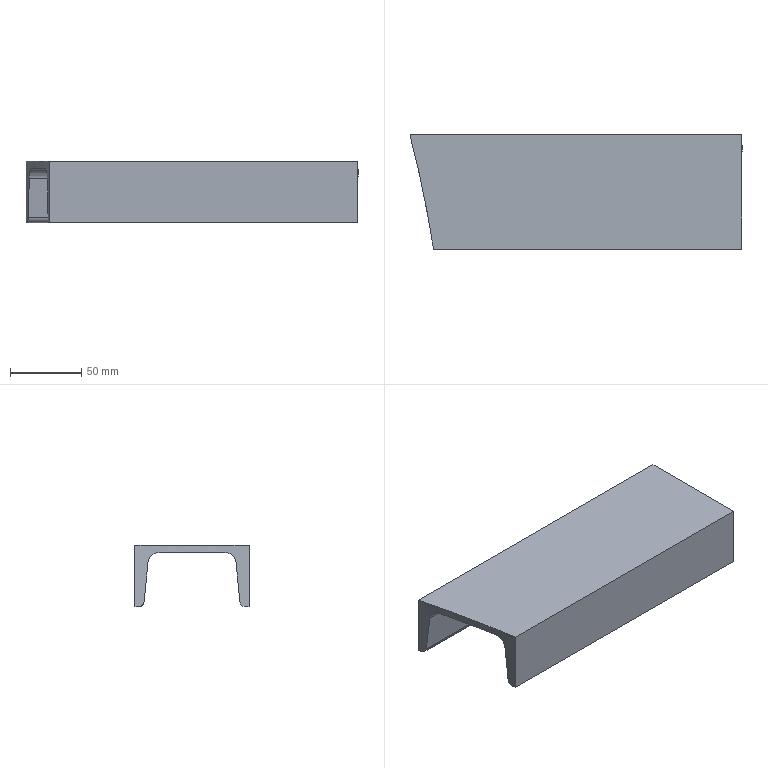Part | SolidWorks | features ICE 2, WeldMemberFeat 1, WeldmentFeature 1 | 1 solid | 14 faces | box 232.5 x 80 x 43 mm | volume 229319 mm3 | plane 9 | cylinder 5 | commonest cylinder face diameters 8 x2 16 x2 1790 x1
STEP:
#1=CARTESIAN_POINT('',(83.602,-77.52,-43.));
#2=VERTEX_POINT('',#1);
#3=CARTESIAN_POINT('',(82.948,-73.54,-39.398));
#4=VERTEX_POINT('',#3);
#5=CARTESIAN_POINT('',(83.602,-77.52,-43.));
#6=CARTESIAN_POINT('',(83.562,-77.274,-43.));
#7=CARTESIAN_POINT('',(83.523,-77.032,-42.978));
#8=CARTESIAN_POINT('',(83.445,-76.555,-42.889));
#9=CARTESIAN_POINT('',(83.407,-76.318,-42.823));
#10=CARTESIAN_POINT('',(83.332,-75.86,-42.648));
#11=CARTESIAN_POINT('',(83.296,-75.642,-42.54));
#12=CARTESIAN_POINT('',(83.227,-75.227,-42.286));
#13=CARTESIAN_POINT('',(83.195,-75.028,-42.138));
#14=CARTESIAN_POINT('',(83.134,-74.663,-41.81));
#15=CARTESIAN_POINT('',(83.107,-74.497,-41.631));
#16=CARTESIAN_POINT('',(83.058,-74.199,-41.242));
#17=CARTESIAN_POINT('',(83.036,-74.065,-41.031));
#18=CARTESIAN_POINT('',(82.998,-73.842,-40.592));
#19=CARTESIAN_POINT('',(82.983,-73.752,-40.365));
#20=CARTESIAN_POINT('',(82.96,-73.613,-39.892));
#21=CARTESIAN_POINT('',(82.952,-73.565,-39.646));
#22=CARTESIAN_POINT('',(82.948,-73.54,-39.398));
#23=B_SPLINE_CURVE_WITH_KNOTS('',3,(#5,#6,#7,#8,#9,#10,#11,#12,#13,#14,#15,#16,#17,#18,#19,#20,#21,#22),.UNSPECIFIED.,.F.,.F.,(4,2,2,2,2,2,2,2,4),(0.,0.0007369,0.001474,0.002211,0.002947,0.003684,0.004421,0.005158,0.005895),.UNSPECIFIED.);
#24=EDGE_CURVE('',#2,#4,#23,.T.);
#25=ORIENTED_EDGE('',*,*,#24,.T.);
#26=CARTESIAN_POINT('',(300.,-73.54,-39.398));
#27=VERTEX_POINT('',#26);
#28=CARTESIAN_POINT('',(300.,-73.54,-39.398));
#29=DIRECTION('',(-1.,0.,0.));
#30=VECTOR('',#29,1000.);
#31=LINE('',#28,#30);
#32=EDGE_CURVE('',#27,#4,#31,.T.);
#33=ORIENTED_EDGE('',*,*,#32,.F.);
#34=CARTESIAN_POINT('',(300.,-77.52,-43.));
#35=VERTEX_POINT('',#34);
#36=CARTESIAN_POINT('',(300.,-77.52,-39.));
#37=DIRECTION('',(-1.,0.,0.));
#38=DIRECTION('',(0.,1.,0.));
#39=AXIS2_PLACEMENT_3D('',#36,#37,#38);
#40=CIRCLE('',#39,4.);
#41=EDGE_CURVE('',#27,#35,#40,.T.);
#42=ORIENTED_EDGE('',*,*,#41,.T.);
#43=CARTESIAN_POINT('',(300.,-77.52,-43.));
#44=DIRECTION('',(-1.,0.,0.));
#45=VECTOR('',#44,1000.);
#46=LINE('',#43,#45);
#47=EDGE_CURVE('',#35,#2,#46,.T.);
#48=ORIENTED_EDGE('',*,*,#47,.T.);
#49=EDGE_LOOP('',(#25,#33,#42,#48));
#50=FACE_OUTER_BOUND('',#49,.T.);
#51=CARTESIAN_POINT('',(300.,-77.52,-39.));
#52=DIRECTION('',(-1.,0.,0.));
#53=DIRECTION('',(0.,0.,1.));
#54=AXIS2_PLACEMENT_3D('',#51,#52,#53);
#55=CYLINDRICAL_SURFACE('',#54,4.);
#56=ADVANCED_FACE('',(#50),#55,.T.);
#57=CARTESIAN_POINT('',(82.491,-70.82,-12.204));
#58=VERTEX_POINT('',#57);
#59=CARTESIAN_POINT('',(82.948,-73.54,-39.398));
#60=CARTESIAN_POINT('',(82.797,-72.633,-30.331));
#61=CARTESIAN_POINT('',(82.645,-71.727,-21.266));
#62=CARTESIAN_POINT('',(82.491,-70.82,-12.204));
#63=(BOUNDED_CURVE()B_SPLINE_CURVE(3,(#59,#60,#61,#62),.UNSPECIFIED.,.F.,.F.)B_SPLINE_CURVE_WITH_KNOTS((4,4),(4.877,4.881),.UNSPECIFIED.)CURVE()GEOMETRIC_REPRESENTATION_ITEM()RATIONAL_B_SPLINE_CURVE((1.,1.,1.,1.))REPRESENTATION_ITEM(''));
#64=EDGE_CURVE('',#4,#58,#63,.T.);
#65=ORIENTED_EDGE('',*,*,#64,.T.);
#66=CARTESIAN_POINT('',(300.,-70.82,-12.204));
#67=VERTEX_POINT('',#66);
#68=CARTESIAN_POINT('',(300.,-70.82,-12.204));
#69=DIRECTION('',(-1.,0.,0.));
#70=VECTOR('',#69,1000.);
#71=LINE('',#68,#70);
#72=EDGE_CURVE('',#67,#58,#71,.T.);
#73=ORIENTED_EDGE('',*,*,#72,.F.);
#74=CARTESIAN_POINT('',(300.,-70.82,-12.204));
#75=DIRECTION('',(0.,-0.0995,-0.995));
#76=VECTOR('',#75,1000.);
#77=LINE('',#74,#76);
#78=EDGE_CURVE('',#67,#27,#77,.T.);
#79=ORIENTED_EDGE('',*,*,#78,.T.);
#80=ORIENTED_EDGE('',*,*,#32,.T.);
#81=EDGE_LOOP('',(#65,#73,#79,#80));
#82=FACE_OUTER_BOUND('',#81,.T.);
#83=CARTESIAN_POINT('',(300.,-70.82,-12.204));
#84=DIRECTION('',(0.,0.995,-0.0995));
#85=DIRECTION('',(0.,0.0995,0.995));
#86=AXIS2_PLACEMENT_3D('',#83,#84,#85);
#87=PLANE('',#86);
#88=ADVANCED_FACE('',(#82),#87,.T.);
#89=CARTESIAN_POINT('',(81.103,-62.86,-5.));
#90=VERTEX_POINT('',#89);
#91=CARTESIAN_POINT('',(82.491,-70.82,-12.204));
#92=CARTESIAN_POINT('',(82.482,-70.771,-11.708));
#93=CARTESIAN_POINT('',(82.466,-70.676,-11.224));
#94=CARTESIAN_POINT('',(82.431,-70.469,-10.517));
#95=CARTESIAN_POINT('',(82.418,-70.389,-10.284));
#96=CARTESIAN_POINT('',(82.387,-70.207,-9.825));
#97=CARTESIAN_POINT('',(82.369,-70.105,-9.598));
#98=CARTESIAN_POINT('',(82.312,-69.769,-8.936));
#99=CARTESIAN_POINT('',(82.267,-69.507,-8.522));
#100=CARTESIAN_POINT('',(82.19,-69.061,-7.939));
#101=CARTESIAN_POINT('',(82.163,-68.902,-7.751));
#102=CARTESIAN_POINT('',(82.105,-68.567,-7.388));
#103=CARTESIAN_POINT('',(82.075,-68.391,-7.215));
#104=CARTESIAN_POINT('',(81.981,-67.844,-6.723));
#105=CARTESIAN_POINT('',(81.913,-67.454,-6.432));
#106=CARTESIAN_POINT('',(81.768,-66.621,-5.922));
#107=CARTESIAN_POINT('',(81.69,-66.176,-5.703));
#108=CARTESIAN_POINT('',(81.53,-65.268,-5.355));
#109=CARTESIAN_POINT('',(81.448,-64.801,-5.224));
#110=CARTESIAN_POINT('',(81.278,-63.842,-5.046));
#111=CARTESIAN_POINT('',(81.19,-63.351,-5.));
#112=CARTESIAN_POINT('',(81.103,-62.86,-5.));
#113=B_SPLINE_CURVE_WITH_KNOTS('',3,(#91,#92,#93,#94,#95,#96,#97,#98,#99,#100,#101,#102,#103,#104,#105,#106,#107,#108,#109,#110,#111,#112),.UNSPECIFIED.,.F.,.F.,(4,2,2,2,2,2,2,2,2,2,4),(0.,0.001475,0.002212,0.00295,0.004425,0.005162,0.0059,0.007375,0.00885,0.01032,0.0118),.UNSPECIFIED.);
#114=EDGE_CURVE('',#58,#90,#113,.T.);
#115=ORIENTED_EDGE('',*,*,#114,.T.);
#116=CARTESIAN_POINT('',(300.,-62.86,-5.));
#117=VERTEX_POINT('',#116);
#118=CARTESIAN_POINT('',(300.,-62.86,-5.));
#119=DIRECTION('',(-1.,0.,0.));
#120=VECTOR('',#119,1000.);
#121=LINE('',#118,#120);
#122=EDGE_CURVE('',#117,#90,#121,.T.);
#123=ORIENTED_EDGE('',*,*,#122,.F.);
#124=CARTESIAN_POINT('',(300.,-62.86,-13.));
#125=DIRECTION('',(1.,0.,0.));
#126=DIRECTION('',(0.,-1.,0.));
#127=AXIS2_PLACEMENT_3D('',#124,#125,#126);
#128=CIRCLE('',#127,8.);
#129=EDGE_CURVE('',#117,#67,#128,.T.);
#130=ORIENTED_EDGE('',*,*,#129,.T.);
#131=ORIENTED_EDGE('',*,*,#72,.T.);
#132=EDGE_LOOP('',(#115,#123,#130,#131));
#133=FACE_OUTER_BOUND('',#132,.T.);
#134=CARTESIAN_POINT('',(300.,-62.86,-13.));
#135=DIRECTION('',(-1.,0.,0.));
#136=DIRECTION('',(0.,0.,1.));
#137=AXIS2_PLACEMENT_3D('',#134,#135,#136);
#138=CYLINDRICAL_SURFACE('',#137,8.);
#139=ADVANCED_FACE('',(#133),#138,.F.);
#140=CARTESIAN_POINT('',(71.68,-17.14,-5.));
#141=VERTEX_POINT('',#140);
#142=CARTESIAN_POINT('',(-799.887,-220.6,-5.));
#143=DIRECTION('',(0.,0.,1.));
#144=DIRECTION('',(0.,1.,0.));
#145=AXIS2_PLACEMENT_3D('',#142,#143,#144);
#146=CIRCLE('',#145,895.);
#147=EDGE_CURVE('',#90,#141,#146,.T.);
#148=ORIENTED_EDGE('',*,*,#147,.T.);
#149=CARTESIAN_POINT('',(300.,-17.14,-5.));
#150=VERTEX_POINT('',#149);
#151=CARTESIAN_POINT('',(300.,-17.14,-5.));
#152=DIRECTION('',(-1.,0.,0.));
#153=VECTOR('',#152,1000.);
#154=LINE('',#151,#153);
#155=EDGE_CURVE('',#150,#141,#154,.T.);
#156=ORIENTED_EDGE('',*,*,#155,.F.);
#157=CARTESIAN_POINT('',(300.,-62.86,-5.));
#158=DIRECTION('',(0.,-1.,0.));
#159=VECTOR('',#158,1000.);
#160=LINE('',#157,#159);
#161=EDGE_CURVE('',#150,#117,#160,.T.);
#162=ORIENTED_EDGE('',*,*,#161,.T.);
#163=ORIENTED_EDGE('',*,*,#122,.T.);
#164=EDGE_LOOP('',(#148,#156,#162,#163));
#165=FACE_OUTER_BOUND('',#164,.T.);
#166=CARTESIAN_POINT('',(300.,-62.86,-5.));
#167=DIRECTION('',(0.,0.,-1.));
#168=DIRECTION('',(0.,1.,0.));
#169=AXIS2_PLACEMENT_3D('',#166,#167,#168);
#170=PLANE('',#169);
#171=ADVANCED_FACE('',(#165),#170,.T.);
#172=CARTESIAN_POINT('',(69.783,-9.18,-12.204));
#173=VERTEX_POINT('',#172);
#174=CARTESIAN_POINT('',(71.68,-17.14,-5.));
#175=CARTESIAN_POINT('',(71.566,-16.651,-5.));
#176=CARTESIAN_POINT('',(71.453,-16.169,-5.044));
#177=CARTESIAN_POINT('',(71.285,-15.458,-5.175));
#178=CARTESIAN_POINT('',(71.23,-15.222,-5.229));
#179=CARTESIAN_POINT('',(71.12,-14.755,-5.36));
#180=CARTESIAN_POINT('',(71.065,-14.522,-5.436));
#181=CARTESIAN_POINT('',(70.902,-13.837,-5.697));
#182=CARTESIAN_POINT('',(70.799,-13.401,-5.911));
#183=CARTESIAN_POINT('',(70.65,-12.78,-6.288));
#184=CARTESIAN_POINT('',(70.602,-12.577,-6.424));
#185=CARTESIAN_POINT('',(70.508,-12.184,-6.715));
#186=CARTESIAN_POINT('',(70.462,-11.992,-6.872));
#187=CARTESIAN_POINT('',(70.33,-11.442,-7.363));
#188=CARTESIAN_POINT('',(70.25,-11.109,-7.721));
#189=CARTESIAN_POINT('',(70.142,-10.66,-8.302));
#190=CARTESIAN_POINT('',(70.107,-10.518,-8.504));
#191=CARTESIAN_POINT('',(70.043,-10.253,-8.922));
#192=CARTESIAN_POINT('',(70.013,-10.129,-9.14));
#193=CARTESIAN_POINT('',(69.931,-9.791,-9.801));
#194=CARTESIAN_POINT('',(69.887,-9.608,-10.259));
#195=CARTESIAN_POINT('',(69.819,-9.327,-11.209));
#196=CARTESIAN_POINT('',(69.795,-9.23,-11.704));
#197=CARTESIAN_POINT('',(69.783,-9.18,-12.204));
#198=B_SPLINE_CURVE_WITH_KNOTS('',3,(#174,#175,#176,#177,#178,#179,#180,#181,#182,#183,#184,#185,#186,#187,#188,#189,#190,#191,#192,#193,#194,#195,#196,#197),.UNSPECIFIED.,.F.,.F.,(4,2,2,2,2,2,2,2,2,2,2,4),(0.,0.001485,0.002228,0.00297,0.004456,0.005198,0.005941,0.007426,0.008169,0.008911,0.0104,0.01188),.UNSPECIFIED.);
#199=EDGE_CURVE('',#141,#173,#198,.T.);
#200=ORIENTED_EDGE('',*,*,#199,.T.);
#201=CARTESIAN_POINT('',(300.,-9.18,-12.204));
#202=VERTEX_POINT('',#201);
#203=CARTESIAN_POINT('',(300.,-9.18,-12.204));
#204=DIRECTION('',(-1.,0.,0.));
#205=VECTOR('',#204,1000.);
#206=LINE('',#203,#205);
#207=EDGE_CURVE('',#202,#173,#206,.T.);
#208=ORIENTED_EDGE('',*,*,#207,.F.);
#209=CARTESIAN_POINT('',(300.,-17.14,-13.));
#210=DIRECTION('',(1.,0.,0.));
#211=DIRECTION('',(0.,1.,0.));
#212=AXIS2_PLACEMENT_3D('',#209,#210,#211);
#213=CIRCLE('',#212,8.);
#214=EDGE_CURVE('',#202,#150,#213,.T.);
#215=ORIENTED_EDGE('',*,*,#214,.T.);
#216=ORIENTED_EDGE('',*,*,#155,.T.);
#217=EDGE_LOOP('',(#200,#208,#215,#216));
#218=FACE_OUTER_BOUND('',#217,.T.);
#219=CARTESIAN_POINT('',(300.,-17.14,-13.));
#220=DIRECTION('',(-1.,0.,0.));
#221=DIRECTION('',(0.,0.,1.));
#222=AXIS2_PLACEMENT_3D('',#219,#220,#221);
#223=CYLINDRICAL_SURFACE('',#222,8.);
#224=ADVANCED_FACE('',(#218),#223,.F.);
#225=CARTESIAN_POINT('',(69.117,-6.46,-39.398));
#226=VERTEX_POINT('',#225);
#227=CARTESIAN_POINT('',(69.783,-9.18,-12.204));
#228=CARTESIAN_POINT('',(69.563,-8.273,-21.272));
#229=CARTESIAN_POINT('',(69.341,-7.366,-30.337));
#230=CARTESIAN_POINT('',(69.117,-6.46,-39.398));
#231=(BOUNDED_CURVE()B_SPLINE_CURVE(3,(#227,#228,#229,#230),.UNSPECIFIED.,.F.,.F.)B_SPLINE_CURVE_WITH_KNOTS((4,4),(1.809,1.812),.UNSPECIFIED.)CURVE()GEOMETRIC_REPRESENTATION_ITEM()RATIONAL_B_SPLINE_CURVE((1.,1.,1.,1.))REPRESENTATION_ITEM(''));
#232=EDGE_CURVE('',#173,#226,#231,.T.);
#233=ORIENTED_EDGE('',*,*,#232,.T.);
#234=CARTESIAN_POINT('',(300.,-6.46,-39.398));
#235=VERTEX_POINT('',#234);
#236=CARTESIAN_POINT('',(300.,-6.46,-39.398));
#237=DIRECTION('',(-1.,0.,0.));
#238=VECTOR('',#237,1000.);
#239=LINE('',#236,#238);
#240=EDGE_CURVE('',#235,#226,#239,.T.);
#241=ORIENTED_EDGE('',*,*,#240,.F.);
#242=CARTESIAN_POINT('',(300.,-9.18,-12.204));
#243=DIRECTION('',(0.,-0.0995,0.995));
#244=VECTOR('',#243,1000.);
#245=LINE('',#242,#244);
#246=EDGE_CURVE('',#235,#202,#245,.T.);
#247=ORIENTED_EDGE('',*,*,#246,.T.);
#248=ORIENTED_EDGE('',*,*,#207,.T.);
#249=EDGE_LOOP('',(#233,#241,#247,#248));
#250=FACE_OUTER_BOUND('',#249,.T.);
#251=CARTESIAN_POINT('',(300.,-9.18,-12.204));
#252=DIRECTION('',(0.,-0.995,-0.0995));
#253=DIRECTION('',(0.,0.0995,-0.995));
#254=AXIS2_PLACEMENT_3D('',#251,#252,#253);
#255=PLANE('',#254);
#256=ADVANCED_FACE('',(#250),#255,.T.);
#257=CARTESIAN_POINT('',(68.127,-2.48,-43.));
#258=VERTEX_POINT('',#257);
#259=CARTESIAN_POINT('',(69.117,-6.46,-39.398));
#260=CARTESIAN_POINT('',(69.111,-6.435,-39.648));
#261=CARTESIAN_POINT('',(69.099,-6.387,-39.892));
#262=CARTESIAN_POINT('',(69.065,-6.248,-40.366));
#263=CARTESIAN_POINT('',(69.042,-6.155,-40.599));
#264=CARTESIAN_POINT('',(68.986,-5.929,-41.041));
#265=CARTESIAN_POINT('',(68.954,-5.797,-41.249));
#266=CARTESIAN_POINT('',(68.88,-5.497,-41.638));
#267=CARTESIAN_POINT('',(68.837,-5.327,-41.82));
#268=CARTESIAN_POINT('',(68.747,-4.962,-42.146));
#269=CARTESIAN_POINT('',(68.698,-4.767,-42.291));
#270=CARTESIAN_POINT('',(68.595,-4.35,-42.544));
#271=CARTESIAN_POINT('',(68.54,-4.128,-42.653));
#272=CARTESIAN_POINT('',(68.427,-3.677,-42.824));
#273=CARTESIAN_POINT('',(68.369,-3.445,-42.89));
#274=CARTESIAN_POINT('',(68.249,-2.967,-42.978));
#275=CARTESIAN_POINT('',(68.188,-2.724,-43.));
#276=CARTESIAN_POINT('',(68.127,-2.48,-43.));
#277=B_SPLINE_CURVE_WITH_KNOTS('',3,(#259,#260,#261,#262,#263,#264,#265,#266,#267,#268,#269,#270,#271,#272,#273,#274,#275,#276),.UNSPECIFIED.,.F.,.F.,(4,2,2,2,2,2,2,2,4),(0.,0.0007434,0.001487,0.00223,0.002974,0.003717,0.004461,0.005204,0.005947),.UNSPECIFIED.);
#278=EDGE_CURVE('',#226,#258,#277,.T.);
#279=ORIENTED_EDGE('',*,*,#278,.T.);
#280=CARTESIAN_POINT('',(300.,-2.48,-43.));
#281=VERTEX_POINT('',#280);
#282=CARTESIAN_POINT('',(300.,-2.48,-43.));
#283=DIRECTION('',(-1.,0.,0.));
#284=VECTOR('',#283,1000.);
#285=LINE('',#282,#284);
#286=EDGE_CURVE('',#281,#258,#285,.T.);
#287=ORIENTED_EDGE('',*,*,#286,.F.);
#288=CARTESIAN_POINT('',(300.,-2.48,-39.));
#289=DIRECTION('',(-1.,0.,0.));
#290=DIRECTION('',(0.,-1.,0.));
#291=AXIS2_PLACEMENT_3D('',#288,#289,#290);
#292=CIRCLE('',#291,4.);
#293=EDGE_CURVE('',#281,#235,#292,.T.);
#294=ORIENTED_EDGE('',*,*,#293,.T.);
#295=ORIENTED_EDGE('',*,*,#240,.T.);
#296=EDGE_LOOP('',(#279,#287,#294,#295));
#297=FACE_OUTER_BOUND('',#296,.T.);
#298=CARTESIAN_POINT('',(300.,-2.48,-39.));
#299=DIRECTION('',(-1.,0.,0.));
#300=DIRECTION('',(0.,0.,1.));
#301=AXIS2_PLACEMENT_3D('',#298,#299,#300);
#302=CYLINDRICAL_SURFACE('',#301,4.);
#303=ADVANCED_FACE('',(#297),#302,.T.);
#304=CARTESIAN_POINT('',(67.5,0.,-43.));
#305=VERTEX_POINT('',#304);
#306=CARTESIAN_POINT('',(-799.887,-220.6,-43.));
#307=DIRECTION('',(0.,0.,1.));
#308=DIRECTION('',(0.,1.,0.));
#309=AXIS2_PLACEMENT_3D('',#306,#307,#308);
#310=CIRCLE('',#309,895.);
#311=EDGE_CURVE('',#258,#305,#310,.T.);
#312=ORIENTED_EDGE('',*,*,#311,.T.);
#313=CARTESIAN_POINT('',(300.,0.,-43.));
#314=VERTEX_POINT('',#313);
#315=CARTESIAN_POINT('',(300.,0.,-43.));
#316=DIRECTION('',(-1.,0.,0.));
#317=VECTOR('',#316,1000.);
#318=LINE('',#315,#317);
#319=EDGE_CURVE('',#314,#305,#318,.T.);
#320=ORIENTED_EDGE('',*,*,#319,.F.);
#321=CARTESIAN_POINT('',(300.,0.,-43.));
#322=DIRECTION('',(0.,-1.,0.));
#323=VECTOR('',#322,1000.);
#324=LINE('',#321,#323);
#325=EDGE_CURVE('',#314,#281,#324,.T.);
#326=ORIENTED_EDGE('',*,*,#325,.T.);
#327=ORIENTED_EDGE('',*,*,#286,.T.);
#328=EDGE_LOOP('',(#312,#320,#326,#327));
#329=FACE_OUTER_BOUND('',#328,.T.);
#330=CARTESIAN_POINT('',(300.,0.,-43.));
#331=DIRECTION('',(0.,0.,-1.));
#332=DIRECTION('',(0.,1.,0.));
#333=AXIS2_PLACEMENT_3D('',#330,#331,#332);
#334=PLANE('',#333);
#335=ADVANCED_FACE('',(#329),#334,.T.);
#336=CARTESIAN_POINT('',(67.5,0.,0.));
#337=VERTEX_POINT('',#336);
#338=CARTESIAN_POINT('',(67.5,0.,-43.001));
#339=DIRECTION('',(0.,0.,1.));
#340=VECTOR('',#339,1000.);
#341=LINE('',#338,#340);
#342=EDGE_CURVE('',#305,#337,#341,.T.);
#343=ORIENTED_EDGE('',*,*,#342,.T.);
#344=CARTESIAN_POINT('',(300.,0.,0.));
#345=VERTEX_POINT('',#344);
#346=CARTESIAN_POINT('',(300.,0.,0.));
#347=DIRECTION('',(-1.,0.,0.));
#348=VECTOR('',#347,1000.);
#349=LINE('',#346,#348);
#350=EDGE_CURVE('',#345,#337,#349,.T.);
#351=ORIENTED_EDGE('',*,*,#350,.F.);
#352=CARTESIAN_POINT('',(300.,0.,-43.));
#353=DIRECTION('',(0.,0.,-1.));
#354=VECTOR('',#353,1000.);
#355=LINE('',#352,#354);
#356=EDGE_CURVE('',#345,#314,#355,.T.);
#357=ORIENTED_EDGE('',*,*,#356,.T.);
#358=ORIENTED_EDGE('',*,*,#319,.T.);
#359=EDGE_LOOP('',(#343,#351,#357,#358));
#360=FACE_OUTER_BOUND('',#359,.T.);
#361=CARTESIAN_POINT('',(300.,0.,-43.));
#362=DIRECTION('',(0.,1.,0.));
#363=DIRECTION('',(0.,0.,1.));
#364=AXIS2_PLACEMENT_3D('',#361,#362,#363);
#365=PLANE('',#364);
#366=ADVANCED_FACE('',(#360),#365,.T.);
#367=CARTESIAN_POINT('',(84.,-80.,0.));
#368=VERTEX_POINT('',#367);
#369=CARTESIAN_POINT('',(-799.887,-220.6,0.));
#370=DIRECTION('',(0.,0.,1.));
#371=DIRECTION('',(1.,0.,0.));
#372=AXIS2_PLACEMENT_3D('',#369,#370,#371);
#373=CIRCLE('',#372,895.);
#374=EDGE_CURVE('',#368,#337,#373,.T.);
#375=ORIENTED_EDGE('',*,*,#374,.F.);
#376=CARTESIAN_POINT('',(300.,-80.,0.));
#377=VERTEX_POINT('',#376);
#378=CARTESIAN_POINT('',(300.,-80.,0.));
#379=DIRECTION('',(-1.,0.,0.));
#380=VECTOR('',#379,1000.);
#381=LINE('',#378,#380);
#382=EDGE_CURVE('',#377,#368,#381,.T.);
#383=ORIENTED_EDGE('',*,*,#382,.F.);
#384=CARTESIAN_POINT('',(300.,-80.,0.));
#385=DIRECTION('',(0.,1.,0.));
#386=VECTOR('',#385,1000.);
#387=LINE('',#384,#386);
#388=EDGE_CURVE('',#377,#345,#387,.T.);
#389=ORIENTED_EDGE('',*,*,#388,.T.);
#390=ORIENTED_EDGE('',*,*,#350,.T.);
#391=EDGE_LOOP('',(#375,#383,#389,#390));
#392=FACE_OUTER_BOUND('',#391,.T.);
#393=CARTESIAN_POINT('',(300.,-80.,0.));
#394=DIRECTION('',(0.,0.,1.));
#395=DIRECTION('',(0.,-1.,0.));
#396=AXIS2_PLACEMENT_3D('',#393,#394,#395);
#397=PLANE('',#396);
#398=ADVANCED_FACE('',(#392),#397,.T.);
#399=CARTESIAN_POINT('',(84.,-80.,-43.));
#400=VERTEX_POINT('',#399);
#401=CARTESIAN_POINT('',(84.,-80.,-43.001));
#402=DIRECTION('',(0.,0.,1.));
#403=VECTOR('',#402,1000.);
#404=LINE('',#401,#403);
#405=EDGE_CURVE('',#400,#368,#404,.T.);
#406=ORIENTED_EDGE('',*,*,#405,.F.);
#407=CARTESIAN_POINT('',(300.,-80.,-43.));
#408=VERTEX_POINT('',#407);
#409=CARTESIAN_POINT('',(300.,-80.,-43.));
#410=DIRECTION('',(-1.,0.,0.));
#411=VECTOR('',#410,1000.);
#412=LINE('',#409,#411);
#413=EDGE_CURVE('',#408,#400,#412,.T.);
#414=ORIENTED_EDGE('',*,*,#413,.F.);
#415=CARTESIAN_POINT('',(300.,-80.,-43.));
#416=DIRECTION('',(0.,0.,1.));
#417=VECTOR('',#416,1000.);
#418=LINE('',#415,#417);
#419=EDGE_CURVE('',#408,#377,#418,.T.);
#420=ORIENTED_EDGE('',*,*,#419,.T.);
#421=ORIENTED_EDGE('',*,*,#382,.T.);
#422=EDGE_LOOP('',(#406,#414,#420,#421));
#423=FACE_OUTER_BOUND('',#422,.T.);
#424=CARTESIAN_POINT('',(300.,-80.,-43.));
#425=DIRECTION('',(0.,-1.,0.));
#426=DIRECTION('',(0.,0.,-1.));
#427=AXIS2_PLACEMENT_3D('',#424,#425,#426);
#428=PLANE('',#427);
#429=ADVANCED_FACE('',(#423),#428,.T.);
#430=CARTESIAN_POINT('',(-799.887,-220.6,-43.));
#431=DIRECTION('',(0.,0.,1.));
#432=DIRECTION('',(0.,1.,0.));
#433=AXIS2_PLACEMENT_3D('',#430,#431,#432);
#434=CIRCLE('',#433,895.);
#435=EDGE_CURVE('',#400,#2,#434,.T.);
#436=ORIENTED_EDGE('',*,*,#435,.T.);
#437=ORIENTED_EDGE('',*,*,#47,.F.);
#438=CARTESIAN_POINT('',(300.,-80.,-43.));
#439=DIRECTION('',(0.,-1.,0.));
#440=VECTOR('',#439,1000.);
#441=LINE('',#438,#440);
#442=EDGE_CURVE('',#35,#408,#441,.T.);
#443=ORIENTED_EDGE('',*,*,#442,.T.);
#444=ORIENTED_EDGE('',*,*,#413,.T.);
#445=EDGE_LOOP('',(#436,#437,#443,#444));
#446=FACE_OUTER_BOUND('',#445,.T.);
#447=CARTESIAN_POINT('',(300.,-80.,-43.));
#448=DIRECTION('',(0.,0.,-1.));
#449=DIRECTION('',(0.,1.,0.));
#450=AXIS2_PLACEMENT_3D('',#447,#448,#449);
#451=PLANE('',#450);
#452=ADVANCED_FACE('',(#446),#451,.T.);
#453=ORIENTED_EDGE('',*,*,#41,.F.);
#454=ORIENTED_EDGE('',*,*,#78,.F.);
#455=ORIENTED_EDGE('',*,*,#129,.F.);
#456=ORIENTED_EDGE('',*,*,#161,.F.);
#457=ORIENTED_EDGE('',*,*,#214,.F.);
#458=ORIENTED_EDGE('',*,*,#246,.F.);
#459=ORIENTED_EDGE('',*,*,#293,.F.);
#460=ORIENTED_EDGE('',*,*,#325,.F.);
#461=ORIENTED_EDGE('',*,*,#356,.F.);
#462=ORIENTED_EDGE('',*,*,#388,.F.);
#463=ORIENTED_EDGE('',*,*,#419,.F.);
#464=ORIENTED_EDGE('',*,*,#442,.F.);
#465=EDGE_LOOP('',(#453,#454,#455,#456,#457,#458,#459,#460,#461,#462,#463,#464));
#466=FACE_OUTER_BOUND('',#465,.T.);
#467=CARTESIAN_POINT('',(300.,-77.52,-39.));
#468=DIRECTION('',(-1.,0.,0.));
#469=DIRECTION('',(0.,1.,0.));
#470=AXIS2_PLACEMENT_3D('',#467,#468,#469);
#471=PLANE('',#470);
#472=ADVANCED_FACE('',(#466),#471,.F.);
#473=ORIENTED_EDGE('',*,*,#278,.F.);
#474=ORIENTED_EDGE('',*,*,#232,.F.);
#475=ORIENTED_EDGE('',*,*,#199,.F.);
#476=ORIENTED_EDGE('',*,*,#147,.F.);
#477=ORIENTED_EDGE('',*,*,#114,.F.);
#478=ORIENTED_EDGE('',*,*,#64,.F.);
#479=ORIENTED_EDGE('',*,*,#24,.F.);
#480=ORIENTED_EDGE('',*,*,#435,.F.);
#481=ORIENTED_EDGE('',*,*,#405,.T.);
#482=ORIENTED_EDGE('',*,*,#374,.T.);
#483=ORIENTED_EDGE('',*,*,#342,.F.);
#484=ORIENTED_EDGE('',*,*,#311,.F.);
#485=EDGE_LOOP('',(#473,#474,#475,#476,#477,#478,#479,#480,#481,#482,#483,#484));
#486=FACE_OUTER_BOUND('',#485,.T.);
#487=CARTESIAN_POINT('',(-799.887,-220.6,-43.001));
#488=DIRECTION('',(0.,0.,1.));
#489=DIRECTION('',(1.,0.,0.));
#490=AXIS2_PLACEMENT_3D('',#487,#488,#489);
#491=CYLINDRICAL_SURFACE('',#490,895.);
#492=ADVANCED_FACE('',(#486),#491,.F.);
#493=CLOSED_SHELL('',(#56,#88,#139,#171,#224,#256,#303,#335,#366,#398,#429,#452,#472,#492));
#494=MANIFOLD_SOLID_BREP('',#493);
#495=CARTESIAN_POINT('',(0.,0.,0.));
#496=DIRECTION('',(0.,0.,1.));
#497=DIRECTION('',(1.,0.,0.));
#498=AXIS2_PLACEMENT_3D('',#495,#496,#497);
#499=(LENGTH_UNIT()NAMED_UNIT(*)SI_UNIT(.MILLI.,.METRE.));
#500=UNCERTAINTY_MEASURE_WITH_UNIT(LENGTH_MEASURE(0.00001),#499,'','');
#501=(NAMED_UNIT(*)PLANE_ANGLE_UNIT()SI_UNIT($,.RADIAN.));
#502=(NAMED_UNIT(*)SI_UNIT($,.STERADIAN.)SOLID_ANGLE_UNIT());
#503=(GEOMETRIC_REPRESENTATION_CONTEXT(3)GLOBAL_UNCERTAINTY_ASSIGNED_CONTEXT((#500))GLOBAL_UNIT_ASSIGNED_CONTEXT((#499,#501,#502))REPRESENTATION_CONTEXT('',''));
#504=ADVANCED_BREP_SHAPE_REPRESENTATION('',(#494,#498),#503);